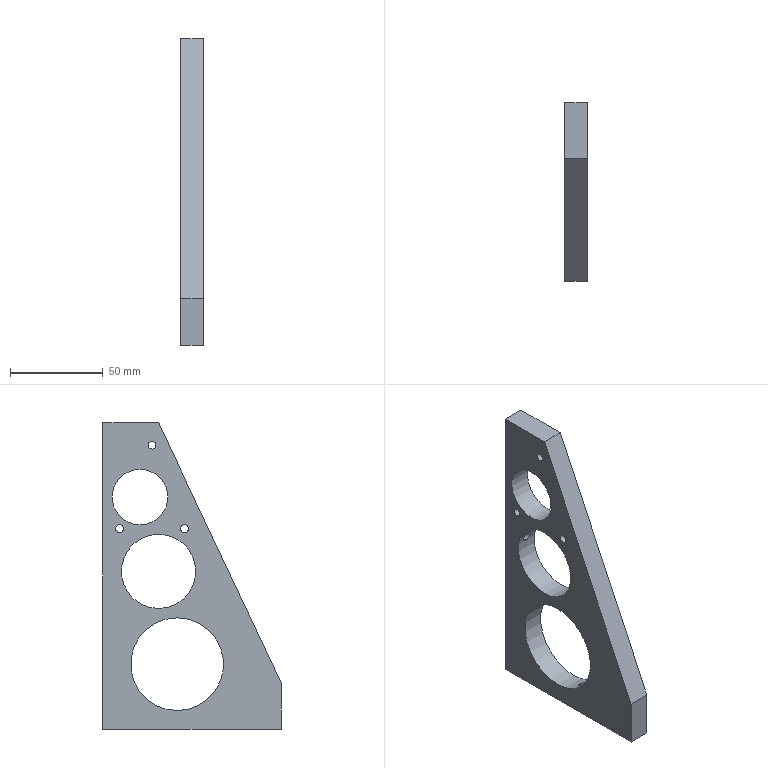Part | NX | 1 solid | 24 faces | box 12 x 96 x 165 mm | volume 85316 mm3 | cylinder 12 | plane 7 | cone 5 | commonest cylinder face diameters 5 x6 4.2 x3 30 x1 40 x1 50 x1
STEP:
#1=CARTESIAN_POINT('',(0.,-3.,-82.5));
#2=VERTEX_POINT('',#1);
#3=CARTESIAN_POINT('',(0.,-5.5,-82.5));
#4=DIRECTION('',(0.,0.,-1.));
#5=DIRECTION('',(0.,1.,0.));
#6=AXIS2_PLACEMENT_3D('',#3,#4,#5);
#7=CIRCLE('',#6,2.5);
#8=EDGE_CURVE('',#2,#2,#7,.T.);
#9=ORIENTED_EDGE('',*,*,#8,.F.);
#10=EDGE_LOOP('',(#9));
#11=FACE_BOUND('',#10,.T.);
#12=CARTESIAN_POINT('',(0.,-38.,-82.5));
#13=VERTEX_POINT('',#12);
#14=CARTESIAN_POINT('',(0.,-40.5,-82.5));
#15=DIRECTION('',(0.,0.,-1.));
#16=DIRECTION('',(0.,1.,0.));
#17=AXIS2_PLACEMENT_3D('',#14,#15,#16);
#18=CIRCLE('',#17,2.5);
#19=EDGE_CURVE('',#13,#13,#18,.T.);
#20=ORIENTED_EDGE('',*,*,#19,.F.);
#21=EDGE_LOOP('',(#20));
#22=FACE_BOUND('',#21,.T.);
#23=CARTESIAN_POINT('',(0.,32.,-82.5));
#24=VERTEX_POINT('',#23);
#25=CARTESIAN_POINT('',(0.,29.5,-82.5));
#26=DIRECTION('',(0.,0.,-1.));
#27=DIRECTION('',(0.,1.,0.));
#28=AXIS2_PLACEMENT_3D('',#25,#26,#27);
#29=CIRCLE('',#28,2.5);
#30=EDGE_CURVE('',#24,#24,#29,.T.);
#31=ORIENTED_EDGE('',*,*,#30,.F.);
#32=EDGE_LOOP('',(#31));
#33=FACE_BOUND('',#32,.T.);
#34=CARTESIAN_POINT('',(-6.,-48.,-82.5));
#35=VERTEX_POINT('',#34);
#36=CARTESIAN_POINT('',(-6.,48.,-82.5));
#37=VERTEX_POINT('',#36);
#38=CARTESIAN_POINT('',(-6.,48.,-82.5));
#39=DIRECTION('',(0.,1.,0.));
#40=VECTOR('',#39,1000.);
#41=LINE('',#38,#40);
#42=EDGE_CURVE('',#35,#37,#41,.T.);
#43=ORIENTED_EDGE('',*,*,#42,.T.);
#44=CARTESIAN_POINT('',(6.,48.,-82.5));
#45=VERTEX_POINT('',#44);
#46=CARTESIAN_POINT('',(6.,48.,-82.5));
#47=DIRECTION('',(-1.,0.,0.));
#48=VECTOR('',#47,1000.);
#49=LINE('',#46,#48);
#50=EDGE_CURVE('',#45,#37,#49,.T.);
#51=ORIENTED_EDGE('',*,*,#50,.F.);
#52=CARTESIAN_POINT('',(6.,-48.,-82.5));
#53=VERTEX_POINT('',#52);
#54=CARTESIAN_POINT('',(6.,48.,-82.5));
#55=DIRECTION('',(0.,1.,0.));
#56=VECTOR('',#55,1000.);
#57=LINE('',#54,#56);
#58=EDGE_CURVE('',#53,#45,#57,.T.);
#59=ORIENTED_EDGE('',*,*,#58,.F.);
#60=CARTESIAN_POINT('',(6.,-48.,-82.5));
#61=DIRECTION('',(-1.,0.,0.));
#62=VECTOR('',#61,1000.);
#63=LINE('',#60,#62);
#64=EDGE_CURVE('',#53,#35,#63,.T.);
#65=ORIENTED_EDGE('',*,*,#64,.T.);
#66=EDGE_LOOP('',(#43,#51,#59,#65));
#67=FACE_BOUND('',#66,.T.);
#68=CARTESIAN_POINT('',(6.,48.,-82.5));
#69=DIRECTION('',(0.,0.,1.));
#70=DIRECTION('',(0.,-1.,0.));
#71=AXIS2_PLACEMENT_3D('',#68,#69,#70);
#72=PLANE('',#71);
#73=ADVANCED_FACE('',(#11,#22,#33,#67),#72,.F.);
#74=CARTESIAN_POINT('',(0.,48.,-55.));
#75=VERTEX_POINT('',#74);
#76=CARTESIAN_POINT('',(0.,48.,-57.5));
#77=DIRECTION('',(0.,1.,0.));
#78=DIRECTION('',(0.,0.,1.));
#79=AXIS2_PLACEMENT_3D('',#76,#77,#78);
#80=CIRCLE('',#79,2.5);
#81=EDGE_CURVE('',#75,#75,#80,.T.);
#82=ORIENTED_EDGE('',*,*,#81,.F.);
#83=EDGE_LOOP('',(#82));
#84=FACE_BOUND('',#83,.T.);
#85=CARTESIAN_POINT('',(0.,48.,10.));
#86=VERTEX_POINT('',#85);
#87=CARTESIAN_POINT('',(0.,48.,7.5));
#88=DIRECTION('',(0.,1.,0.));
#89=DIRECTION('',(0.,0.,1.));
#90=AXIS2_PLACEMENT_3D('',#87,#88,#89);
#91=CIRCLE('',#90,2.5);
#92=EDGE_CURVE('',#86,#86,#91,.T.);
#93=ORIENTED_EDGE('',*,*,#92,.F.);
#94=EDGE_LOOP('',(#93));
#95=FACE_BOUND('',#94,.T.);
#96=CARTESIAN_POINT('',(0.,48.,75.));
#97=VERTEX_POINT('',#96);
#98=CARTESIAN_POINT('',(0.,48.,72.5));
#99=DIRECTION('',(0.,1.,0.));
#100=DIRECTION('',(0.,0.,1.));
#101=AXIS2_PLACEMENT_3D('',#98,#99,#100);
#102=CIRCLE('',#101,2.5);
#103=EDGE_CURVE('',#97,#97,#102,.T.);
#104=ORIENTED_EDGE('',*,*,#103,.F.);
#105=EDGE_LOOP('',(#104));
#106=FACE_BOUND('',#105,.T.);
#107=CARTESIAN_POINT('',(-6.,48.,82.5));
#108=VERTEX_POINT('',#107);
#109=CARTESIAN_POINT('',(-6.,48.,82.5));
#110=DIRECTION('',(0.,0.,1.));
#111=VECTOR('',#110,1000.);
#112=LINE('',#109,#111);
#113=EDGE_CURVE('',#37,#108,#112,.T.);
#114=ORIENTED_EDGE('',*,*,#113,.T.);
#115=CARTESIAN_POINT('',(6.,48.,82.5));
#116=VERTEX_POINT('',#115);
#117=CARTESIAN_POINT('',(6.,48.,82.5));
#118=DIRECTION('',(-1.,0.,0.));
#119=VECTOR('',#118,1000.);
#120=LINE('',#117,#119);
#121=EDGE_CURVE('',#116,#108,#120,.T.);
#122=ORIENTED_EDGE('',*,*,#121,.F.);
#123=CARTESIAN_POINT('',(6.,48.,82.5));
#124=DIRECTION('',(0.,0.,1.));
#125=VECTOR('',#124,1000.);
#126=LINE('',#123,#125);
#127=EDGE_CURVE('',#45,#116,#126,.T.);
#128=ORIENTED_EDGE('',*,*,#127,.F.);
#129=ORIENTED_EDGE('',*,*,#50,.T.);
#130=EDGE_LOOP('',(#114,#122,#128,#129));
#131=FACE_BOUND('',#130,.T.);
#132=CARTESIAN_POINT('',(6.,48.,82.5));
#133=DIRECTION('',(0.,-1.,0.));
#134=DIRECTION('',(0.,0.,-1.));
#135=AXIS2_PLACEMENT_3D('',#132,#133,#134);
#136=PLANE('',#135);
#137=ADVANCED_FACE('',(#84,#95,#106,#131),#136,.F.);
#138=CARTESIAN_POINT('',(-6.,18.,82.5));
#139=VERTEX_POINT('',#138);
#140=CARTESIAN_POINT('',(-6.,48.,82.5));
#141=DIRECTION('',(0.,-1.,0.));
#142=VECTOR('',#141,1000.);
#143=LINE('',#140,#142);
#144=EDGE_CURVE('',#108,#139,#143,.T.);
#145=ORIENTED_EDGE('',*,*,#144,.T.);
#146=CARTESIAN_POINT('',(6.,18.,82.5));
#147=VERTEX_POINT('',#146);
#148=CARTESIAN_POINT('',(-14.,18.,82.5));
#149=DIRECTION('',(1.,0.,0.));
#150=VECTOR('',#149,1000.);
#151=LINE('',#148,#150);
#152=EDGE_CURVE('',#139,#147,#151,.T.);
#153=ORIENTED_EDGE('',*,*,#152,.T.);
#154=CARTESIAN_POINT('',(6.,48.,82.5));
#155=DIRECTION('',(0.,-1.,0.));
#156=VECTOR('',#155,1000.);
#157=LINE('',#154,#156);
#158=EDGE_CURVE('',#116,#147,#157,.T.);
#159=ORIENTED_EDGE('',*,*,#158,.F.);
#160=ORIENTED_EDGE('',*,*,#121,.T.);
#161=EDGE_LOOP('',(#145,#153,#159,#160));
#162=FACE_BOUND('',#161,.T.);
#163=CARTESIAN_POINT('',(6.,48.,82.5));
#164=DIRECTION('',(0.,0.,-1.));
#165=DIRECTION('',(0.,1.,0.));
#166=AXIS2_PLACEMENT_3D('',#163,#164,#165);
#167=PLANE('',#166);
#168=ADVANCED_FACE('',(#162),#167,.F.);
#169=CARTESIAN_POINT('',(6.,-48.,-57.5));
#170=VERTEX_POINT('',#169);
#171=CARTESIAN_POINT('',(6.,-48.,82.5));
#172=DIRECTION('',(0.,0.,-1.));
#173=VECTOR('',#172,1000.);
#174=LINE('',#171,#173);
#175=EDGE_CURVE('',#170,#53,#174,.T.);
#176=ORIENTED_EDGE('',*,*,#175,.F.);
#177=CARTESIAN_POINT('',(-6.,-48.,-57.5));
#178=VERTEX_POINT('',#177);
#179=CARTESIAN_POINT('',(-14.,-48.,-57.5));
#180=DIRECTION('',(1.,0.,0.));
#181=VECTOR('',#180,1000.);
#182=LINE('',#179,#181);
#183=EDGE_CURVE('',#178,#170,#182,.T.);
#184=ORIENTED_EDGE('',*,*,#183,.F.);
#185=CARTESIAN_POINT('',(-6.,-48.,82.5));
#186=DIRECTION('',(0.,0.,-1.));
#187=VECTOR('',#186,1000.);
#188=LINE('',#185,#187);
#189=EDGE_CURVE('',#178,#35,#188,.T.);
#190=ORIENTED_EDGE('',*,*,#189,.T.);
#191=ORIENTED_EDGE('',*,*,#64,.F.);
#192=EDGE_LOOP('',(#176,#184,#190,#191));
#193=FACE_BOUND('',#192,.T.);
#194=CARTESIAN_POINT('',(6.,-48.,82.5));
#195=DIRECTION('',(0.,1.,0.));
#196=DIRECTION('',(0.,0.,1.));
#197=AXIS2_PLACEMENT_3D('',#194,#195,#196);
#198=PLANE('',#197);
#199=ADVANCED_FACE('',(#193),#198,.F.);
#200=CARTESIAN_POINT('',(6.,4.,23.4));
#201=VERTEX_POINT('',#200);
#202=CARTESIAN_POINT('',(6.,4.,25.5));
#203=DIRECTION('',(1.,0.,0.));
#204=DIRECTION('',(0.,0.,-1.));
#205=AXIS2_PLACEMENT_3D('',#202,#203,#204);
#206=CIRCLE('',#205,2.1);
#207=EDGE_CURVE('',#201,#201,#206,.T.);
#208=ORIENTED_EDGE('',*,*,#207,.F.);
#209=EDGE_LOOP('',(#208));
#210=FACE_BOUND('',#209,.T.);
#211=CARTESIAN_POINT('',(6.,39.,23.4));
#212=VERTEX_POINT('',#211);
#213=CARTESIAN_POINT('',(6.,39.,25.5));
#214=DIRECTION('',(1.,0.,0.));
#215=DIRECTION('',(0.,0.,-1.));
#216=AXIS2_PLACEMENT_3D('',#213,#214,#215);
#217=CIRCLE('',#216,2.1);
#218=EDGE_CURVE('',#212,#212,#217,.T.);
#219=ORIENTED_EDGE('',*,*,#218,.F.);
#220=EDGE_LOOP('',(#219));
#221=FACE_BOUND('',#220,.T.);
#222=CARTESIAN_POINT('',(6.,21.5,68.4));
#223=VERTEX_POINT('',#222);
#224=CARTESIAN_POINT('',(6.,21.5,70.5));
#225=DIRECTION('',(1.,0.,0.));
#226=DIRECTION('',(0.,0.,-1.));
#227=AXIS2_PLACEMENT_3D('',#224,#225,#226);
#228=CIRCLE('',#227,2.1);
#229=EDGE_CURVE('',#223,#223,#228,.T.);
#230=ORIENTED_EDGE('',*,*,#229,.F.);
#231=EDGE_LOOP('',(#230));
#232=FACE_BOUND('',#231,.T.);
#233=CARTESIAN_POINT('',(6.,28.,57.5));
#234=VERTEX_POINT('',#233);
#235=CARTESIAN_POINT('',(6.,28.,42.5));
#236=DIRECTION('',(-1.,0.,0.));
#237=DIRECTION('',(0.,0.,1.));
#238=AXIS2_PLACEMENT_3D('',#235,#236,#237);
#239=CIRCLE('',#238,15.);
#240=EDGE_CURVE('',#234,#234,#239,.T.);
#241=ORIENTED_EDGE('',*,*,#240,.T.);
#242=EDGE_LOOP('',(#241));
#243=FACE_BOUND('',#242,.T.);
#244=CARTESIAN_POINT('',(6.,18.,22.5));
#245=VERTEX_POINT('',#244);
#246=CARTESIAN_POINT('',(6.,18.,2.5));
#247=DIRECTION('',(-1.,0.,0.));
#248=DIRECTION('',(0.,0.,1.));
#249=AXIS2_PLACEMENT_3D('',#246,#247,#248);
#250=CIRCLE('',#249,20.);
#251=EDGE_CURVE('',#245,#245,#250,.T.);
#252=ORIENTED_EDGE('',*,*,#251,.T.);
#253=EDGE_LOOP('',(#252));
#254=FACE_BOUND('',#253,.T.);
#255=CARTESIAN_POINT('',(6.,8.,-22.5));
#256=VERTEX_POINT('',#255);
#257=CARTESIAN_POINT('',(6.,8.,-47.5));
#258=DIRECTION('',(-1.,0.,0.));
#259=DIRECTION('',(0.,0.,1.));
#260=AXIS2_PLACEMENT_3D('',#257,#258,#259);
#261=CIRCLE('',#260,25.);
#262=EDGE_CURVE('',#256,#256,#261,.T.);
#263=ORIENTED_EDGE('',*,*,#262,.T.);
#264=EDGE_LOOP('',(#263));
#265=FACE_BOUND('',#264,.T.);
#266=CARTESIAN_POINT('',(6.,-48.,-57.5));
#267=DIRECTION('',(0.,0.4264,0.9045));
#268=VECTOR('',#267,1000.);
#269=LINE('',#266,#268);
#270=EDGE_CURVE('',#170,#147,#269,.T.);
#271=ORIENTED_EDGE('',*,*,#270,.F.);
#272=ORIENTED_EDGE('',*,*,#175,.T.);
#273=ORIENTED_EDGE('',*,*,#58,.T.);
#274=ORIENTED_EDGE('',*,*,#127,.T.);
#275=ORIENTED_EDGE('',*,*,#158,.T.);
#276=EDGE_LOOP('',(#271,#272,#273,#274,#275));
#277=FACE_BOUND('',#276,.T.);
#278=CARTESIAN_POINT('',(6.,0.,0.));
#279=DIRECTION('',(1.,0.,0.));
#280=DIRECTION('',(0.,0.,-1.));
#281=AXIS2_PLACEMENT_3D('',#278,#279,#280);
#282=PLANE('',#281);
#283=ADVANCED_FACE('',(#210,#221,#232,#243,#254,#265,#277),#282,.T.);
#284=CARTESIAN_POINT('',(-6.,4.,23.4));
#285=VERTEX_POINT('',#284);
#286=CARTESIAN_POINT('',(-6.,4.,25.5));
#287=DIRECTION('',(1.,0.,0.));
#288=DIRECTION('',(0.,0.,-1.));
#289=AXIS2_PLACEMENT_3D('',#286,#287,#288);
#290=CIRCLE('',#289,2.1);
#291=EDGE_CURVE('',#285,#285,#290,.T.);
#292=ORIENTED_EDGE('',*,*,#291,.T.);
#293=EDGE_LOOP('',(#292));
#294=FACE_BOUND('',#293,.T.);
#295=CARTESIAN_POINT('',(-6.,39.,23.4));
#296=VERTEX_POINT('',#295);
#297=CARTESIAN_POINT('',(-6.,39.,25.5));
#298=DIRECTION('',(1.,0.,0.));
#299=DIRECTION('',(0.,0.,-1.));
#300=AXIS2_PLACEMENT_3D('',#297,#298,#299);
#301=CIRCLE('',#300,2.1);
#302=EDGE_CURVE('',#296,#296,#301,.T.);
#303=ORIENTED_EDGE('',*,*,#302,.T.);
#304=EDGE_LOOP('',(#303));
#305=FACE_BOUND('',#304,.T.);
#306=CARTESIAN_POINT('',(-6.,21.5,68.4));
#307=VERTEX_POINT('',#306);
#308=CARTESIAN_POINT('',(-6.,21.5,70.5));
#309=DIRECTION('',(1.,0.,0.));
#310=DIRECTION('',(0.,0.,-1.));
#311=AXIS2_PLACEMENT_3D('',#308,#309,#310);
#312=CIRCLE('',#311,2.1);
#313=EDGE_CURVE('',#307,#307,#312,.T.);
#314=ORIENTED_EDGE('',*,*,#313,.T.);
#315=EDGE_LOOP('',(#314));
#316=FACE_BOUND('',#315,.T.);
#317=CARTESIAN_POINT('',(-6.,28.,57.5));
#318=VERTEX_POINT('',#317);
#319=CARTESIAN_POINT('',(-6.,28.,42.5));
#320=DIRECTION('',(-1.,0.,0.));
#321=DIRECTION('',(0.,0.,1.));
#322=AXIS2_PLACEMENT_3D('',#319,#320,#321);
#323=CIRCLE('',#322,15.);
#324=EDGE_CURVE('',#318,#318,#323,.T.);
#325=ORIENTED_EDGE('',*,*,#324,.F.);
#326=EDGE_LOOP('',(#325));
#327=FACE_BOUND('',#326,.T.);
#328=CARTESIAN_POINT('',(-6.,18.,22.5));
#329=VERTEX_POINT('',#328);
#330=CARTESIAN_POINT('',(-6.,18.,2.5));
#331=DIRECTION('',(-1.,0.,0.));
#332=DIRECTION('',(0.,0.,1.));
#333=AXIS2_PLACEMENT_3D('',#330,#331,#332);
#334=CIRCLE('',#333,20.);
#335=EDGE_CURVE('',#329,#329,#334,.T.);
#336=ORIENTED_EDGE('',*,*,#335,.F.);
#337=EDGE_LOOP('',(#336));
#338=FACE_BOUND('',#337,.T.);
#339=CARTESIAN_POINT('',(-6.,8.,-22.5));
#340=VERTEX_POINT('',#339);
#341=CARTESIAN_POINT('',(-6.,8.,-47.5));
#342=DIRECTION('',(-1.,0.,0.));
#343=DIRECTION('',(0.,0.,1.));
#344=AXIS2_PLACEMENT_3D('',#341,#342,#343);
#345=CIRCLE('',#344,25.);
#346=EDGE_CURVE('',#340,#340,#345,.T.);
#347=ORIENTED_EDGE('',*,*,#346,.F.);
#348=EDGE_LOOP('',(#347));
#349=FACE_BOUND('',#348,.T.);
#350=ORIENTED_EDGE('',*,*,#189,.F.);
#351=CARTESIAN_POINT('',(-6.,-17.094,8.059));
#352=DIRECTION('',(0.,0.4264,0.9045));
#353=VECTOR('',#352,1000.);
#354=LINE('',#351,#353);
#355=EDGE_CURVE('',#178,#139,#354,.T.);
#356=ORIENTED_EDGE('',*,*,#355,.T.);
#357=ORIENTED_EDGE('',*,*,#144,.F.);
#358=ORIENTED_EDGE('',*,*,#113,.F.);
#359=ORIENTED_EDGE('',*,*,#42,.F.);
#360=EDGE_LOOP('',(#350,#356,#357,#358,#359));
#361=FACE_BOUND('',#360,.T.);
#362=CARTESIAN_POINT('',(-6.,0.,0.));
#363=DIRECTION('',(1.,0.,0.));
#364=DIRECTION('',(0.,0.,-1.));
#365=AXIS2_PLACEMENT_3D('',#362,#363,#364);
#366=PLANE('',#365);
#367=ADVANCED_FACE('',(#294,#305,#316,#327,#338,#349,#361),#366,.F.);
#368=ORIENTED_EDGE('',*,*,#183,.T.);
#369=ORIENTED_EDGE('',*,*,#270,.T.);
#370=ORIENTED_EDGE('',*,*,#152,.F.);
#371=ORIENTED_EDGE('',*,*,#355,.F.);
#372=EDGE_LOOP('',(#368,#369,#370,#371));
#373=FACE_BOUND('',#372,.T.);
#374=CARTESIAN_POINT('',(-14.,-48.,-57.5));
#375=DIRECTION('',(0.,0.9045,-0.4264));
#376=DIRECTION('',(0.,0.4264,0.9045));
#377=AXIS2_PLACEMENT_3D('',#374,#375,#376);
#378=PLANE('',#377);
#379=ADVANCED_FACE('',(#373),#378,.F.);
#380=CARTESIAN_POINT('',(0.,29.5,-65.998));
#381=VERTEX_POINT('',#380);
#382=VERTEX_LOOP('',#381);
#383=FACE_BOUND('',#382,.T.);
#384=CARTESIAN_POINT('',(0.,32.,-67.5));
#385=VERTEX_POINT('',#384);
#386=CARTESIAN_POINT('',(0.,29.5,-67.5));
#387=DIRECTION('',(0.,0.,-1.));
#388=DIRECTION('',(0.,1.,0.));
#389=AXIS2_PLACEMENT_3D('',#386,#387,#388);
#390=CIRCLE('',#389,2.5);
#391=EDGE_CURVE('',#385,#385,#390,.T.);
#392=ORIENTED_EDGE('',*,*,#391,.T.);
#393=EDGE_LOOP('',(#392));
#394=FACE_BOUND('',#393,.T.);
#395=CARTESIAN_POINT('',(0.,29.5,-67.5));
#396=DIRECTION('',(0.,0.,-1.));
#397=DIRECTION('',(0.,1.,0.));
#398=AXIS2_PLACEMENT_3D('',#395,#396,#397);
#399=CONICAL_SURFACE('',#398,2.5,1.03);
#400=ADVANCED_FACE('',(#383,#394),#399,.F.);
#401=ORIENTED_EDGE('',*,*,#391,.F.);
#402=EDGE_LOOP('',(#401));
#403=FACE_BOUND('',#402,.T.);
#404=ORIENTED_EDGE('',*,*,#30,.T.);
#405=EDGE_LOOP('',(#404));
#406=FACE_BOUND('',#405,.T.);
#407=CARTESIAN_POINT('',(0.,29.5,-82.5));
#408=DIRECTION('',(0.,0.,-1.));
#409=DIRECTION('',(0.,1.,0.));
#410=AXIS2_PLACEMENT_3D('',#407,#408,#409);
#411=CYLINDRICAL_SURFACE('',#410,2.5);
#412=ADVANCED_FACE('',(#403,#406),#411,.F.);
#413=CARTESIAN_POINT('',(0.,-40.5,-65.998));
#414=VERTEX_POINT('',#413);
#415=VERTEX_LOOP('',#414);
#416=FACE_BOUND('',#415,.T.);
#417=CARTESIAN_POINT('',(0.,-38.,-67.5));
#418=VERTEX_POINT('',#417);
#419=CARTESIAN_POINT('',(0.,-40.5,-67.5));
#420=DIRECTION('',(0.,0.,-1.));
#421=DIRECTION('',(0.,1.,0.));
#422=AXIS2_PLACEMENT_3D('',#419,#420,#421);
#423=CIRCLE('',#422,2.5);
#424=EDGE_CURVE('',#418,#418,#423,.T.);
#425=ORIENTED_EDGE('',*,*,#424,.T.);
#426=EDGE_LOOP('',(#425));
#427=FACE_BOUND('',#426,.T.);
#428=CARTESIAN_POINT('',(0.,-40.5,-67.5));
#429=DIRECTION('',(0.,0.,-1.));
#430=DIRECTION('',(0.,1.,0.));
#431=AXIS2_PLACEMENT_3D('',#428,#429,#430);
#432=CONICAL_SURFACE('',#431,2.5,1.03);
#433=ADVANCED_FACE('',(#416,#427),#432,.F.);
#434=ORIENTED_EDGE('',*,*,#424,.F.);
#435=EDGE_LOOP('',(#434));
#436=FACE_BOUND('',#435,.T.);
#437=ORIENTED_EDGE('',*,*,#19,.T.);
#438=EDGE_LOOP('',(#437));
#439=FACE_BOUND('',#438,.T.);
#440=CARTESIAN_POINT('',(0.,-40.5,-82.5));
#441=DIRECTION('',(0.,0.,-1.));
#442=DIRECTION('',(0.,1.,0.));
#443=AXIS2_PLACEMENT_3D('',#440,#441,#442);
#444=CYLINDRICAL_SURFACE('',#443,2.5);
#445=ADVANCED_FACE('',(#436,#439),#444,.F.);
#446=CARTESIAN_POINT('',(2.,-7.,-67.5));
#447=VERTEX_POINT('',#446);
#448=CARTESIAN_POINT('',(-2.,-7.,-67.5));
#449=VERTEX_POINT('',#448);
#450=CARTESIAN_POINT('',(0.,-5.5,-67.5));
#451=DIRECTION('',(0.,0.,-1.));
#452=DIRECTION('',(0.,1.,0.));
#453=AXIS2_PLACEMENT_3D('',#450,#451,#452);
#454=CIRCLE('',#453,2.5);
#455=EDGE_CURVE('',#447,#449,#454,.T.);
#456=ORIENTED_EDGE('',*,*,#455,.T.);
#457=CARTESIAN_POINT('',(-2.,-7.,-67.5));
#458=CARTESIAN_POINT('',(-1.387,-7.265,-67.301));
#459=CARTESIAN_POINT('',(-0.004321,-7.612,-67.025));
#460=CARTESIAN_POINT('',(1.385,-7.266,-67.3));
#461=CARTESIAN_POINT('',(2.,-7.,-67.5));
#462=B_SPLINE_CURVE_WITH_KNOTS('',3,(#457,#458,#459,#460,#461),.UNSPECIFIED.,.F.,.F.,(4,1,4),(0.0004924,0.002582,0.004671),.UNSPECIFIED.);
#463=EDGE_CURVE('',#449,#447,#462,.T.);
#464=ORIENTED_EDGE('',*,*,#463,.T.);
#465=EDGE_LOOP('',(#456,#464));
#466=FACE_BOUND('',#465,.T.);
#467=CARTESIAN_POINT('',(0.,-5.5,-67.5));
#468=DIRECTION('',(0.,0.,-1.));
#469=DIRECTION('',(0.,1.,0.));
#470=AXIS2_PLACEMENT_3D('',#467,#468,#469);
#471=CONICAL_SURFACE('',#470,2.5,1.03);
#472=ADVANCED_FACE('',(#466),#471,.F.);
#473=ORIENTED_EDGE('',*,*,#455,.F.);
#474=CARTESIAN_POINT('',(2.,-7.,-67.5));
#475=CARTESIAN_POINT('',(2.531,-6.291,-68.031));
#476=CARTESIAN_POINT('',(2.721,-4.905,-68.953));
#477=CARTESIAN_POINT('',(1.546,-3.345,-69.784));
#478=CARTESIAN_POINT('',(0.01827,-2.832,-70.03));
#479=CARTESIAN_POINT('',(-1.522,-3.326,-69.794));
#480=CARTESIAN_POINT('',(-2.724,-4.892,-68.962));
#481=CARTESIAN_POINT('',(-2.532,-6.29,-68.032));
#482=CARTESIAN_POINT('',(-2.,-7.,-67.5));
#483=B_SPLINE_CURVE_WITH_KNOTS('',3,(#474,#475,#476,#477,#478,#479,#480,#481,#482),.UNSPECIFIED.,.F.,.F.,(4,1,1,1,1,1,4),(0.,0.003045,0.004568,0.006091,0.007614,0.009136,0.01218),.UNSPECIFIED.);
#484=EDGE_CURVE('',#447,#449,#483,.T.);
#485=ORIENTED_EDGE('',*,*,#484,.T.);
#486=EDGE_LOOP('',(#473,#485));
#487=FACE_BOUND('',#486,.T.);
#488=ORIENTED_EDGE('',*,*,#8,.T.);
#489=EDGE_LOOP('',(#488));
#490=FACE_BOUND('',#489,.T.);
#491=CARTESIAN_POINT('',(0.,-5.5,-82.5));
#492=DIRECTION('',(0.,0.,-1.));
#493=DIRECTION('',(0.,1.,0.));
#494=AXIS2_PLACEMENT_3D('',#491,#492,#493);
#495=CYLINDRICAL_SURFACE('',#494,2.5);
#496=ADVANCED_FACE('',(#487,#490),#495,.F.);
#497=CARTESIAN_POINT('',(0.,31.498,72.5));
#498=VERTEX_POINT('',#497);
#499=VERTEX_LOOP('',#498);
#500=FACE_BOUND('',#499,.T.);
#501=CARTESIAN_POINT('',(0.,33.,75.));
#502=VERTEX_POINT('',#501);
#503=CARTESIAN_POINT('',(0.,33.,72.5));
#504=DIRECTION('',(0.,1.,0.));
#505=DIRECTION('',(0.,0.,1.));
#506=AXIS2_PLACEMENT_3D('',#503,#504,#505);
#507=CIRCLE('',#506,2.5);
#508=EDGE_CURVE('',#502,#502,#507,.T.);
#509=ORIENTED_EDGE('',*,*,#508,.T.);
#510=EDGE_LOOP('',(#509));
#511=FACE_BOUND('',#510,.T.);
#512=CARTESIAN_POINT('',(0.,33.,72.5));
#513=DIRECTION('',(0.,1.,0.));
#514=DIRECTION('',(0.,0.,1.));
#515=AXIS2_PLACEMENT_3D('',#512,#513,#514);
#516=CONICAL_SURFACE('',#515,2.5,1.03);
#517=ADVANCED_FACE('',(#500,#511),#516,.F.);
#518=ORIENTED_EDGE('',*,*,#508,.F.);
#519=EDGE_LOOP('',(#518));
#520=FACE_BOUND('',#519,.T.);
#521=ORIENTED_EDGE('',*,*,#103,.T.);
#522=EDGE_LOOP('',(#521));
#523=FACE_BOUND('',#522,.T.);
#524=CARTESIAN_POINT('',(0.,48.,72.5));
#525=DIRECTION('',(0.,1.,0.));
#526=DIRECTION('',(0.,0.,1.));
#527=AXIS2_PLACEMENT_3D('',#524,#525,#526);
#528=CYLINDRICAL_SURFACE('',#527,2.5);
#529=ADVANCED_FACE('',(#520,#523),#528,.F.);
#530=CARTESIAN_POINT('',(0.,36.54,10.));
#531=VERTEX_POINT('',#530);
#532=CARTESIAN_POINT('',(1.973,36.78,9.434));
#533=CARTESIAN_POINT('',(0.00007015,36.421,10.283));
#534=CARTESIAN_POINT('',(-1.973,36.78,9.434));
#535=CARTESIAN_POINT('',(-2.757,37.395,7.543));
#536=CARTESIAN_POINT('',(-1.996,37.783,5.568));
#537=CARTESIAN_POINT('',(-0.0003875,37.873,4.717));
#538=CARTESIAN_POINT('',(1.993,37.783,5.564));
#539=CARTESIAN_POINT('',(2.758,37.395,7.543));
#540=CARTESIAN_POINT('',(1.973,36.78,9.434));
#541=CARTESIAN_POINT('',(0.00007015,36.421,10.283));
#542=CARTESIAN_POINT('',(-1.973,36.78,9.434));
#543=B_SPLINE_CURVE_WITH_KNOTS('',3,(#532,#533,#534,#535,#536,#537,#538,#539,#540,#541,#542),.UNSPECIFIED.,.T.,.F.,(1,1,1,1,1,1,1,1,1,1,1,1,1,1,1),(-0.005967,-0.003978,-0.001989,0.,0.001989,0.003978,0.005967,0.007956,0.009945,0.01193,0.01392,0.01591,0.0179,0.01989,0.02188),.UNSPECIFIED.);
#544=EDGE_CURVE('',#531,#531,#543,.T.);
#545=ORIENTED_EDGE('',*,*,#544,.T.);
#546=EDGE_LOOP('',(#545));
#547=FACE_BOUND('',#546,.T.);
#548=ORIENTED_EDGE('',*,*,#92,.T.);
#549=EDGE_LOOP('',(#548));
#550=FACE_BOUND('',#549,.T.);
#551=CARTESIAN_POINT('',(0.,48.,7.5));
#552=DIRECTION('',(0.,1.,0.));
#553=DIRECTION('',(0.,0.,1.));
#554=AXIS2_PLACEMENT_3D('',#551,#552,#553);
#555=CYLINDRICAL_SURFACE('',#554,2.5);
#556=ADVANCED_FACE('',(#547,#550),#555,.F.);
#557=CARTESIAN_POINT('',(0.,31.498,-57.5));
#558=VERTEX_POINT('',#557);
#559=VERTEX_LOOP('',#558);
#560=FACE_BOUND('',#559,.T.);
#561=CARTESIAN_POINT('',(0.,33.,-55.));
#562=VERTEX_POINT('',#561);
#563=CARTESIAN_POINT('',(0.,33.,-57.5));
#564=DIRECTION('',(0.,1.,0.));
#565=DIRECTION('',(0.,0.,1.));
#566=AXIS2_PLACEMENT_3D('',#563,#564,#565);
#567=CIRCLE('',#566,2.5);
#568=EDGE_CURVE('',#562,#562,#567,.T.);
#569=ORIENTED_EDGE('',*,*,#568,.T.);
#570=EDGE_LOOP('',(#569));
#571=FACE_BOUND('',#570,.T.);
#572=CARTESIAN_POINT('',(0.,33.,-57.5));
#573=DIRECTION('',(0.,1.,0.));
#574=DIRECTION('',(0.,0.,1.));
#575=AXIS2_PLACEMENT_3D('',#572,#573,#574);
#576=CONICAL_SURFACE('',#575,2.5,1.03);
#577=ADVANCED_FACE('',(#560,#571),#576,.F.);
#578=ORIENTED_EDGE('',*,*,#568,.F.);
#579=EDGE_LOOP('',(#578));
#580=FACE_BOUND('',#579,.T.);
#581=ORIENTED_EDGE('',*,*,#81,.T.);
#582=EDGE_LOOP('',(#581));
#583=FACE_BOUND('',#582,.T.);
#584=CARTESIAN_POINT('',(0.,48.,-57.5));
#585=DIRECTION('',(0.,1.,0.));
#586=DIRECTION('',(0.,0.,1.));
#587=AXIS2_PLACEMENT_3D('',#584,#585,#586);
#588=CYLINDRICAL_SURFACE('',#587,2.5);
#589=ADVANCED_FACE('',(#580,#583),#588,.F.);
#590=ORIENTED_EDGE('',*,*,#346,.T.);
#591=EDGE_LOOP('',(#590));
#592=FACE_BOUND('',#591,.T.);
#593=ORIENTED_EDGE('',*,*,#262,.F.);
#594=EDGE_LOOP('',(#593));
#595=FACE_BOUND('',#594,.T.);
#596=ORIENTED_EDGE('',*,*,#484,.F.);
#597=ORIENTED_EDGE('',*,*,#463,.F.);
#598=EDGE_LOOP('',(#596,#597));
#599=FACE_BOUND('',#598,.T.);
#600=CARTESIAN_POINT('',(6.,8.,-47.5));
#601=DIRECTION('',(-1.,0.,0.));
#602=DIRECTION('',(0.,0.,1.));
#603=AXIS2_PLACEMENT_3D('',#600,#601,#602);
#604=CYLINDRICAL_SURFACE('',#603,25.);
#605=ADVANCED_FACE('',(#592,#595,#599),#604,.F.);
#606=ORIENTED_EDGE('',*,*,#335,.T.);
#607=EDGE_LOOP('',(#606));
#608=FACE_BOUND('',#607,.T.);
#609=ORIENTED_EDGE('',*,*,#251,.F.);
#610=EDGE_LOOP('',(#609));
#611=FACE_BOUND('',#610,.T.);
#612=ORIENTED_EDGE('',*,*,#544,.F.);
#613=EDGE_LOOP('',(#612));
#614=FACE_BOUND('',#613,.T.);
#615=CARTESIAN_POINT('',(6.,18.,2.5));
#616=DIRECTION('',(-1.,0.,0.));
#617=DIRECTION('',(0.,0.,1.));
#618=AXIS2_PLACEMENT_3D('',#615,#616,#617);
#619=CYLINDRICAL_SURFACE('',#618,20.);
#620=ADVANCED_FACE('',(#608,#611,#614),#619,.F.);
#621=ORIENTED_EDGE('',*,*,#240,.F.);
#622=EDGE_LOOP('',(#621));
#623=FACE_BOUND('',#622,.T.);
#624=ORIENTED_EDGE('',*,*,#324,.T.);
#625=EDGE_LOOP('',(#624));
#626=FACE_BOUND('',#625,.T.);
#627=CARTESIAN_POINT('',(6.,28.,42.5));
#628=DIRECTION('',(-1.,0.,0.));
#629=DIRECTION('',(0.,0.,1.));
#630=AXIS2_PLACEMENT_3D('',#627,#628,#629);
#631=CYLINDRICAL_SURFACE('',#630,15.);
#632=ADVANCED_FACE('',(#623,#626),#631,.F.);
#633=ORIENTED_EDGE('',*,*,#229,.T.);
#634=EDGE_LOOP('',(#633));
#635=FACE_BOUND('',#634,.T.);
#636=ORIENTED_EDGE('',*,*,#313,.F.);
#637=EDGE_LOOP('',(#636));
#638=FACE_BOUND('',#637,.T.);
#639=CARTESIAN_POINT('',(6.,21.5,70.5));
#640=DIRECTION('',(1.,0.,0.));
#641=DIRECTION('',(0.,0.,-1.));
#642=AXIS2_PLACEMENT_3D('',#639,#640,#641);
#643=CYLINDRICAL_SURFACE('',#642,2.1);
#644=ADVANCED_FACE('',(#635,#638),#643,.F.);
#645=ORIENTED_EDGE('',*,*,#218,.T.);
#646=EDGE_LOOP('',(#645));
#647=FACE_BOUND('',#646,.T.);
#648=ORIENTED_EDGE('',*,*,#302,.F.);
#649=EDGE_LOOP('',(#648));
#650=FACE_BOUND('',#649,.T.);
#651=CARTESIAN_POINT('',(6.,39.,25.5));
#652=DIRECTION('',(1.,0.,0.));
#653=DIRECTION('',(0.,0.,-1.));
#654=AXIS2_PLACEMENT_3D('',#651,#652,#653);
#655=CYLINDRICAL_SURFACE('',#654,2.1);
#656=ADVANCED_FACE('',(#647,#650),#655,.F.);
#657=ORIENTED_EDGE('',*,*,#207,.T.);
#658=EDGE_LOOP('',(#657));
#659=FACE_BOUND('',#658,.T.);
#660=ORIENTED_EDGE('',*,*,#291,.F.);
#661=EDGE_LOOP('',(#660));
#662=FACE_BOUND('',#661,.T.);
#663=CARTESIAN_POINT('',(6.,4.,25.5));
#664=DIRECTION('',(1.,0.,0.));
#665=DIRECTION('',(0.,0.,-1.));
#666=AXIS2_PLACEMENT_3D('',#663,#664,#665);
#667=CYLINDRICAL_SURFACE('',#666,2.1);
#668=ADVANCED_FACE('',(#659,#662),#667,.F.);
#669=CLOSED_SHELL('',(#73,#137,#168,#199,#283,#367,#379,#400,#412,#433,#445,#472,#496,#517,#529,#556,#577,#589,#605,#620,#632,#644,#656,#668));
#670=MANIFOLD_SOLID_BREP('',#669);
#671=(LENGTH_UNIT()NAMED_UNIT(*)SI_UNIT(.MILLI.,.METRE.));
#672=UNCERTAINTY_MEASURE_WITH_UNIT(LENGTH_MEASURE(0.0508),#671,'','');
#673=(NAMED_UNIT(*)PLANE_ANGLE_UNIT()SI_UNIT($,.RADIAN.));
#674=(NAMED_UNIT(*)SI_UNIT($,.STERADIAN.)SOLID_ANGLE_UNIT());
#675=(GEOMETRIC_REPRESENTATION_CONTEXT(3)GLOBAL_UNCERTAINTY_ASSIGNED_CONTEXT((#672))GLOBAL_UNIT_ASSIGNED_CONTEXT((#671,#673,#674))REPRESENTATION_CONTEXT('',''));
#676=ADVANCED_BREP_SHAPE_REPRESENTATION('',(#670),#675);